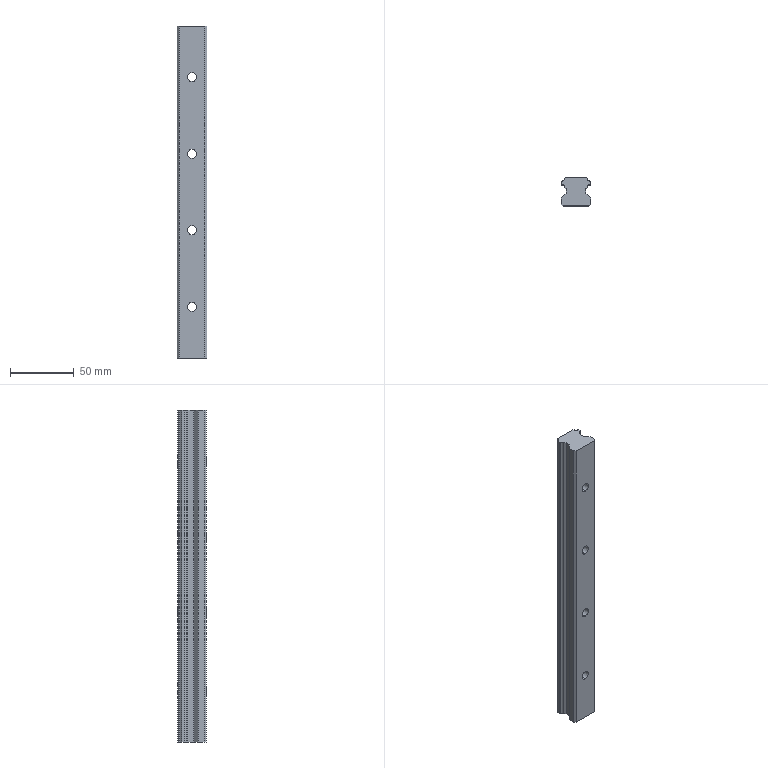Part | SolidWorks | features ICE 2, BaseBody 1, HoleWzd 1, LPattern 1 | 1 solid | 48 faces | box 23 x 22 x 260 mm | volume 107500 mm3 | plane 26 | cylinder 22 | commonest cylinder face diameters 7 x8 11 x8 3.5 x6
STEP:
#1=CARTESIAN_POINT('',(0.,-9.,-134.5));
#2=VERTEX_POINT('',#1);
#3=CARTESIAN_POINT('',(0.,-9.,-123.5));
#4=VERTEX_POINT('',#3);
#5=CARTESIAN_POINT('',(0.,-9.,-129.));
#6=DIRECTION('',(0.,1.,0.));
#7=DIRECTION('',(0.,0.,1.));
#8=AXIS2_PLACEMENT_3D('',#5,#6,#7);
#9=CIRCLE('',#8,5.5);
#10=EDGE_CURVE('',#2,#4,#9,.T.);
#11=ORIENTED_EDGE('',*,*,#10,.F.);
#12=CARTESIAN_POINT('',(0.,0.,-134.5));
#13=VERTEX_POINT('',#12);
#14=CARTESIAN_POINT('',(0.,0.,-134.5));
#15=DIRECTION('',(0.,1.,0.));
#16=VECTOR('',#15,1000.);
#17=LINE('',#14,#16);
#18=EDGE_CURVE('',#2,#13,#17,.T.);
#19=ORIENTED_EDGE('',*,*,#18,.T.);
#20=CARTESIAN_POINT('',(0.,0.,-123.5));
#21=VERTEX_POINT('',#20);
#22=CARTESIAN_POINT('',(0.,0.,-129.));
#23=DIRECTION('',(0.,1.,0.));
#24=DIRECTION('',(0.,0.,1.));
#25=AXIS2_PLACEMENT_3D('',#22,#23,#24);
#26=CIRCLE('',#25,5.5);
#27=EDGE_CURVE('',#13,#21,#26,.T.);
#28=ORIENTED_EDGE('',*,*,#27,.T.);
#29=CARTESIAN_POINT('',(0.,0.,-123.5));
#30=DIRECTION('',(0.,1.,0.));
#31=VECTOR('',#30,1000.);
#32=LINE('',#29,#31);
#33=EDGE_CURVE('',#4,#21,#32,.T.);
#34=ORIENTED_EDGE('',*,*,#33,.F.);
#35=EDGE_LOOP('',(#11,#19,#28,#34));
#36=FACE_OUTER_BOUND('',#35,.T.);
#37=CARTESIAN_POINT('',(0.,0.,-129.));
#38=DIRECTION('',(0.,1.,0.));
#39=DIRECTION('',(0.,0.,1.));
#40=AXIS2_PLACEMENT_3D('',#37,#38,#39);
#41=CYLINDRICAL_SURFACE('',#40,5.5);
#42=ADVANCED_FACE('',(#36),#41,.F.);
#43=CARTESIAN_POINT('',(0.,-22.,-125.5));
#44=VERTEX_POINT('',#43);
#45=CARTESIAN_POINT('',(0.,-22.,-132.5));
#46=VERTEX_POINT('',#45);
#47=CARTESIAN_POINT('',(0.,-22.,-129.));
#48=DIRECTION('',(0.,-1.,0.));
#49=DIRECTION('',(0.,0.,-1.));
#50=AXIS2_PLACEMENT_3D('',#47,#48,#49);
#51=CIRCLE('',#50,3.5);
#52=EDGE_CURVE('',#44,#46,#51,.T.);
#53=ORIENTED_EDGE('',*,*,#52,.T.);
#54=CARTESIAN_POINT('',(0.,-9.,-132.5));
#55=VERTEX_POINT('',#54);
#56=CARTESIAN_POINT('',(0.,0.,-132.5));
#57=DIRECTION('',(0.,1.,0.));
#58=VECTOR('',#57,1000.);
#59=LINE('',#56,#58);
#60=EDGE_CURVE('',#46,#55,#59,.T.);
#61=ORIENTED_EDGE('',*,*,#60,.T.);
#62=CARTESIAN_POINT('',(0.,-9.,-125.5));
#63=VERTEX_POINT('',#62);
#64=CARTESIAN_POINT('',(0.,-9.,-129.));
#65=DIRECTION('',(0.,1.,0.));
#66=DIRECTION('',(0.,0.,1.));
#67=AXIS2_PLACEMENT_3D('',#64,#65,#66);
#68=CIRCLE('',#67,3.5);
#69=EDGE_CURVE('',#55,#63,#68,.T.);
#70=ORIENTED_EDGE('',*,*,#69,.T.);
#71=CARTESIAN_POINT('',(0.,0.,-125.5));
#72=DIRECTION('',(0.,1.,0.));
#73=VECTOR('',#72,1000.);
#74=LINE('',#71,#73);
#75=EDGE_CURVE('',#44,#63,#74,.T.);
#76=ORIENTED_EDGE('',*,*,#75,.F.);
#77=EDGE_LOOP('',(#53,#61,#70,#76));
#78=FACE_OUTER_BOUND('',#77,.T.);
#79=CARTESIAN_POINT('',(0.,0.,-129.));
#80=DIRECTION('',(0.,1.,0.));
#81=DIRECTION('',(0.,0.,1.));
#82=AXIS2_PLACEMENT_3D('',#79,#80,#81);
#83=CYLINDRICAL_SURFACE('',#82,3.5);
#84=ADVANCED_FACE('',(#78),#83,.F.);
#85=CARTESIAN_POINT('',(0.,-9.,-74.5));
#86=VERTEX_POINT('',#85);
#87=CARTESIAN_POINT('',(0.,-9.,-63.5));
#88=VERTEX_POINT('',#87);
#89=CARTESIAN_POINT('',(0.,-9.,-69.));
#90=DIRECTION('',(0.,1.,0.));
#91=DIRECTION('',(0.,0.,1.));
#92=AXIS2_PLACEMENT_3D('',#89,#90,#91);
#93=CIRCLE('',#92,5.5);
#94=EDGE_CURVE('',#86,#88,#93,.T.);
#95=ORIENTED_EDGE('',*,*,#94,.F.);
#96=CARTESIAN_POINT('',(0.,0.,-74.5));
#97=VERTEX_POINT('',#96);
#98=CARTESIAN_POINT('',(0.,0.,-74.5));
#99=DIRECTION('',(0.,1.,0.));
#100=VECTOR('',#99,1000.);
#101=LINE('',#98,#100);
#102=EDGE_CURVE('',#86,#97,#101,.T.);
#103=ORIENTED_EDGE('',*,*,#102,.T.);
#104=CARTESIAN_POINT('',(0.,0.,-63.5));
#105=VERTEX_POINT('',#104);
#106=CARTESIAN_POINT('',(0.,0.,-69.));
#107=DIRECTION('',(0.,1.,0.));
#108=DIRECTION('',(0.,0.,1.));
#109=AXIS2_PLACEMENT_3D('',#106,#107,#108);
#110=CIRCLE('',#109,5.5);
#111=EDGE_CURVE('',#97,#105,#110,.T.);
#112=ORIENTED_EDGE('',*,*,#111,.T.);
#113=CARTESIAN_POINT('',(0.,0.,-63.5));
#114=DIRECTION('',(0.,1.,0.));
#115=VECTOR('',#114,1000.);
#116=LINE('',#113,#115);
#117=EDGE_CURVE('',#88,#105,#116,.T.);
#118=ORIENTED_EDGE('',*,*,#117,.F.);
#119=EDGE_LOOP('',(#95,#103,#112,#118));
#120=FACE_OUTER_BOUND('',#119,.T.);
#121=CARTESIAN_POINT('',(0.,0.,-69.));
#122=DIRECTION('',(0.,1.,0.));
#123=DIRECTION('',(0.,0.,1.));
#124=AXIS2_PLACEMENT_3D('',#121,#122,#123);
#125=CYLINDRICAL_SURFACE('',#124,5.5);
#126=ADVANCED_FACE('',(#120),#125,.F.);
#127=CARTESIAN_POINT('',(0.,-22.,-65.5));
#128=VERTEX_POINT('',#127);
#129=CARTESIAN_POINT('',(0.,-22.,-72.5));
#130=VERTEX_POINT('',#129);
#131=CARTESIAN_POINT('',(0.,-22.,-69.));
#132=DIRECTION('',(0.,-1.,0.));
#133=DIRECTION('',(0.,0.,-1.));
#134=AXIS2_PLACEMENT_3D('',#131,#132,#133);
#135=CIRCLE('',#134,3.5);
#136=EDGE_CURVE('',#128,#130,#135,.T.);
#137=ORIENTED_EDGE('',*,*,#136,.T.);
#138=CARTESIAN_POINT('',(0.,-9.,-72.5));
#139=VERTEX_POINT('',#138);
#140=CARTESIAN_POINT('',(0.,0.,-72.5));
#141=DIRECTION('',(0.,1.,0.));
#142=VECTOR('',#141,1000.);
#143=LINE('',#140,#142);
#144=EDGE_CURVE('',#130,#139,#143,.T.);
#145=ORIENTED_EDGE('',*,*,#144,.T.);
#146=CARTESIAN_POINT('',(0.,-9.,-65.5));
#147=VERTEX_POINT('',#146);
#148=CARTESIAN_POINT('',(0.,-9.,-69.));
#149=DIRECTION('',(0.,1.,0.));
#150=DIRECTION('',(0.,0.,1.));
#151=AXIS2_PLACEMENT_3D('',#148,#149,#150);
#152=CIRCLE('',#151,3.5);
#153=EDGE_CURVE('',#139,#147,#152,.T.);
#154=ORIENTED_EDGE('',*,*,#153,.T.);
#155=CARTESIAN_POINT('',(0.,0.,-65.5));
#156=DIRECTION('',(0.,1.,0.));
#157=VECTOR('',#156,1000.);
#158=LINE('',#155,#157);
#159=EDGE_CURVE('',#128,#147,#158,.T.);
#160=ORIENTED_EDGE('',*,*,#159,.F.);
#161=EDGE_LOOP('',(#137,#145,#154,#160));
#162=FACE_OUTER_BOUND('',#161,.T.);
#163=CARTESIAN_POINT('',(0.,0.,-69.));
#164=DIRECTION('',(0.,1.,0.));
#165=DIRECTION('',(0.,0.,1.));
#166=AXIS2_PLACEMENT_3D('',#163,#164,#165);
#167=CYLINDRICAL_SURFACE('',#166,3.5);
#168=ADVANCED_FACE('',(#162),#167,.F.);
#169=CARTESIAN_POINT('',(0.,-9.,-5.5));
#170=VERTEX_POINT('',#169);
#171=CARTESIAN_POINT('',(0.,-9.,-12.5));
#172=VERTEX_POINT('',#171);
#173=CARTESIAN_POINT('',(0.,-9.,-9.));
#174=DIRECTION('',(0.,-1.,0.));
#175=DIRECTION('',(0.,0.,-1.));
#176=AXIS2_PLACEMENT_3D('',#173,#174,#175);
#177=CIRCLE('',#176,3.5);
#178=EDGE_CURVE('',#170,#172,#177,.T.);
#179=ORIENTED_EDGE('',*,*,#178,.F.);
#180=CARTESIAN_POINT('',(0.,-22.,-5.5));
#181=VERTEX_POINT('',#180);
#182=CARTESIAN_POINT('',(0.,-22.,-5.5));
#183=DIRECTION('',(0.,-1.,0.));
#184=VECTOR('',#183,1000.);
#185=LINE('',#182,#184);
#186=EDGE_CURVE('',#170,#181,#185,.T.);
#187=ORIENTED_EDGE('',*,*,#186,.T.);
#188=CARTESIAN_POINT('',(0.,-22.,-12.5));
#189=VERTEX_POINT('',#188);
#190=CARTESIAN_POINT('',(0.,-22.,-9.));
#191=DIRECTION('',(0.,1.,0.));
#192=DIRECTION('',(0.,0.,-1.));
#193=AXIS2_PLACEMENT_3D('',#190,#191,#192);
#194=CIRCLE('',#193,3.5);
#195=EDGE_CURVE('',#189,#181,#194,.T.);
#196=ORIENTED_EDGE('',*,*,#195,.F.);
#197=CARTESIAN_POINT('',(0.,-22.,-12.5));
#198=DIRECTION('',(0.,-1.,0.));
#199=VECTOR('',#198,1000.);
#200=LINE('',#197,#199);
#201=EDGE_CURVE('',#172,#189,#200,.T.);
#202=ORIENTED_EDGE('',*,*,#201,.F.);
#203=EDGE_LOOP('',(#179,#187,#196,#202));
#204=FACE_OUTER_BOUND('',#203,.T.);
#205=CARTESIAN_POINT('',(0.,-22.,-9.));
#206=DIRECTION('',(0.,-1.,0.));
#207=DIRECTION('',(0.,0.,-1.));
#208=AXIS2_PLACEMENT_3D('',#205,#206,#207);
#209=CYLINDRICAL_SURFACE('',#208,3.5);
#210=ADVANCED_FACE('',(#204),#209,.F.);
#211=CARTESIAN_POINT('',(0.,-9.,54.5));
#212=VERTEX_POINT('',#211);
#213=CARTESIAN_POINT('',(0.,-9.,47.5));
#214=VERTEX_POINT('',#213);
#215=CARTESIAN_POINT('',(0.,-9.,51.));
#216=DIRECTION('',(0.,-1.,0.));
#217=DIRECTION('',(0.,0.,-1.));
#218=AXIS2_PLACEMENT_3D('',#215,#216,#217);
#219=CIRCLE('',#218,3.5);
#220=EDGE_CURVE('',#212,#214,#219,.T.);
#221=ORIENTED_EDGE('',*,*,#220,.F.);
#222=CARTESIAN_POINT('',(0.,-22.,54.5));
#223=VERTEX_POINT('',#222);
#224=CARTESIAN_POINT('',(0.,-22.,54.5));
#225=DIRECTION('',(0.,-1.,0.));
#226=VECTOR('',#225,1000.);
#227=LINE('',#224,#226);
#228=EDGE_CURVE('',#212,#223,#227,.T.);
#229=ORIENTED_EDGE('',*,*,#228,.T.);
#230=CARTESIAN_POINT('',(0.,-22.,47.5));
#231=VERTEX_POINT('',#230);
#232=CARTESIAN_POINT('',(0.,-22.,51.));
#233=DIRECTION('',(0.,1.,0.));
#234=DIRECTION('',(0.,0.,-1.));
#235=AXIS2_PLACEMENT_3D('',#232,#233,#234);
#236=CIRCLE('',#235,3.5);
#237=EDGE_CURVE('',#231,#223,#236,.T.);
#238=ORIENTED_EDGE('',*,*,#237,.F.);
#239=CARTESIAN_POINT('',(0.,-22.,47.5));
#240=DIRECTION('',(0.,-1.,0.));
#241=VECTOR('',#240,1000.);
#242=LINE('',#239,#241);
#243=EDGE_CURVE('',#214,#231,#242,.T.);
#244=ORIENTED_EDGE('',*,*,#243,.F.);
#245=EDGE_LOOP('',(#221,#229,#238,#244));
#246=FACE_OUTER_BOUND('',#245,.T.);
#247=CARTESIAN_POINT('',(0.,-22.,51.));
#248=DIRECTION('',(0.,-1.,0.));
#249=DIRECTION('',(0.,0.,-1.));
#250=AXIS2_PLACEMENT_3D('',#247,#248,#249);
#251=CYLINDRICAL_SURFACE('',#250,3.5);
#252=ADVANCED_FACE('',(#246),#251,.F.);
#253=CARTESIAN_POINT('',(-9.017,-7.063,-169.));
#254=VERTEX_POINT('',#253);
#255=CARTESIAN_POINT('',(-11.079,-5.341,-169.));
#256=VERTEX_POINT('',#255);
#257=CARTESIAN_POINT('',(-10.767,-7.063,-169.));
#258=DIRECTION('',(0.,0.,1.));
#259=DIRECTION('',(-1.,0.,0.));
#260=AXIS2_PLACEMENT_3D('',#257,#258,#259);
#261=CIRCLE('',#260,1.75);
#262=EDGE_CURVE('',#254,#256,#261,.T.);
#263=ORIENTED_EDGE('',*,*,#262,.F.);
#264=CARTESIAN_POINT('',(-9.017,-7.063,91.));
#265=VERTEX_POINT('',#264);
#266=CARTESIAN_POINT('',(-9.017,-7.063,71.));
#267=DIRECTION('',(0.,0.,1.));
#268=VECTOR('',#267,1000.);
#269=LINE('',#266,#268);
#270=EDGE_CURVE('',#254,#265,#269,.T.);
#271=ORIENTED_EDGE('',*,*,#270,.T.);
#272=CARTESIAN_POINT('',(-11.079,-5.341,91.));
#273=VERTEX_POINT('',#272);
#274=CARTESIAN_POINT('',(-10.767,-7.063,91.));
#275=DIRECTION('',(0.,0.,-1.));
#276=DIRECTION('',(1.,0.,0.));
#277=AXIS2_PLACEMENT_3D('',#274,#275,#276);
#278=CIRCLE('',#277,1.75);
#279=EDGE_CURVE('',#273,#265,#278,.T.);
#280=ORIENTED_EDGE('',*,*,#279,.F.);
#281=CARTESIAN_POINT('',(-11.079,-5.341,71.));
#282=DIRECTION('',(0.,0.,1.));
#283=VECTOR('',#282,1000.);
#284=LINE('',#281,#283);
#285=EDGE_CURVE('',#256,#273,#284,.T.);
#286=ORIENTED_EDGE('',*,*,#285,.F.);
#287=EDGE_LOOP('',(#263,#271,#280,#286));
#288=FACE_OUTER_BOUND('',#287,.T.);
#289=CARTESIAN_POINT('',(-10.767,-7.063,71.));
#290=DIRECTION('',(0.,0.,1.));
#291=DIRECTION('',(1.,0.,0.));
#292=AXIS2_PLACEMENT_3D('',#289,#290,#291);
#293=CYLINDRICAL_SURFACE('',#292,1.75);
#294=ADVANCED_FACE('',(#288),#293,.F.);
#295=CARTESIAN_POINT('',(-9.022,-0.9324,-169.));
#296=VERTEX_POINT('',#295);
#297=CARTESIAN_POINT('',(-9.047,-0.6384,-169.));
#298=VERTEX_POINT('',#297);
#299=CARTESIAN_POINT('',(-10.772,-0.9324,-169.));
#300=DIRECTION('',(0.,0.,1.));
#301=DIRECTION('',(-1.,0.,0.));
#302=AXIS2_PLACEMENT_3D('',#299,#300,#301);
#303=CIRCLE('',#302,1.75);
#304=EDGE_CURVE('',#296,#298,#303,.T.);
#305=ORIENTED_EDGE('',*,*,#304,.F.);
#306=CARTESIAN_POINT('',(-9.022,-0.9324,91.));
#307=VERTEX_POINT('',#306);
#308=CARTESIAN_POINT('',(-9.022,-0.9324,71.));
#309=DIRECTION('',(0.,0.,1.));
#310=VECTOR('',#309,1000.);
#311=LINE('',#308,#310);
#312=EDGE_CURVE('',#296,#307,#311,.T.);
#313=ORIENTED_EDGE('',*,*,#312,.T.);
#314=CARTESIAN_POINT('',(-9.047,-0.6384,91.));
#315=VERTEX_POINT('',#314);
#316=CARTESIAN_POINT('',(-10.772,-0.9324,91.));
#317=DIRECTION('',(0.,0.,-1.));
#318=DIRECTION('',(1.,0.,0.));
#319=AXIS2_PLACEMENT_3D('',#316,#317,#318);
#320=CIRCLE('',#319,1.75);
#321=EDGE_CURVE('',#315,#307,#320,.T.);
#322=ORIENTED_EDGE('',*,*,#321,.F.);
#323=CARTESIAN_POINT('',(-9.047,-0.6384,71.));
#324=DIRECTION('',(0.,0.,1.));
#325=VECTOR('',#324,1000.);
#326=LINE('',#323,#325);
#327=EDGE_CURVE('',#298,#315,#326,.T.);
#328=ORIENTED_EDGE('',*,*,#327,.F.);
#329=EDGE_LOOP('',(#305,#313,#322,#328));
#330=FACE_OUTER_BOUND('',#329,.T.);
#331=CARTESIAN_POINT('',(-10.772,-0.9324,71.));
#332=DIRECTION('',(0.,0.,1.));
#333=DIRECTION('',(1.,0.,0.));
#334=AXIS2_PLACEMENT_3D('',#331,#332,#333);
#335=CYLINDRICAL_SURFACE('',#334,1.75);
#336=ADVANCED_FACE('',(#330),#335,.F.);
#337=CARTESIAN_POINT('',(0.,-9.,-14.5));
#338=VERTEX_POINT('',#337);
#339=CARTESIAN_POINT('',(0.,-9.,-3.5));
#340=VERTEX_POINT('',#339);
#341=CARTESIAN_POINT('',(0.,-9.,-9.));
#342=DIRECTION('',(0.,1.,0.));
#343=DIRECTION('',(0.,0.,1.));
#344=AXIS2_PLACEMENT_3D('',#341,#342,#343);
#345=CIRCLE('',#344,5.5);
#346=EDGE_CURVE('',#338,#340,#345,.T.);
#347=ORIENTED_EDGE('',*,*,#346,.F.);
#348=CARTESIAN_POINT('',(0.,0.,-14.5));
#349=VERTEX_POINT('',#348);
#350=CARTESIAN_POINT('',(0.,0.,-14.5));
#351=DIRECTION('',(0.,1.,0.));
#352=VECTOR('',#351,1000.);
#353=LINE('',#350,#352);
#354=EDGE_CURVE('',#338,#349,#353,.T.);
#355=ORIENTED_EDGE('',*,*,#354,.T.);
#356=CARTESIAN_POINT('',(0.,0.,-3.5));
#357=VERTEX_POINT('',#356);
#358=CARTESIAN_POINT('',(0.,0.,-9.));
#359=DIRECTION('',(0.,-1.,0.));
#360=DIRECTION('',(0.,0.,1.));
#361=AXIS2_PLACEMENT_3D('',#358,#359,#360);
#362=CIRCLE('',#361,5.5);
#363=EDGE_CURVE('',#357,#349,#362,.T.);
#364=ORIENTED_EDGE('',*,*,#363,.F.);
#365=CARTESIAN_POINT('',(0.,0.,-3.5));
#366=DIRECTION('',(0.,1.,0.));
#367=VECTOR('',#366,1000.);
#368=LINE('',#365,#367);
#369=EDGE_CURVE('',#340,#357,#368,.T.);
#370=ORIENTED_EDGE('',*,*,#369,.F.);
#371=EDGE_LOOP('',(#347,#355,#364,#370));
#372=FACE_OUTER_BOUND('',#371,.T.);
#373=CARTESIAN_POINT('',(0.,0.,-9.));
#374=DIRECTION('',(0.,1.,0.));
#375=DIRECTION('',(0.,0.,1.));
#376=AXIS2_PLACEMENT_3D('',#373,#374,#375);
#377=CYLINDRICAL_SURFACE('',#376,5.5);
#378=ADVANCED_FACE('',(#372),#377,.F.);
#379=CARTESIAN_POINT('',(0.,-9.,45.5));
#380=VERTEX_POINT('',#379);
#381=CARTESIAN_POINT('',(0.,-9.,56.5));
#382=VERTEX_POINT('',#381);
#383=CARTESIAN_POINT('',(0.,-9.,51.));
#384=DIRECTION('',(0.,1.,0.));
#385=DIRECTION('',(0.,0.,1.));
#386=AXIS2_PLACEMENT_3D('',#383,#384,#385);
#387=CIRCLE('',#386,5.5);
#388=EDGE_CURVE('',#380,#382,#387,.T.);
#389=ORIENTED_EDGE('',*,*,#388,.F.);
#390=CARTESIAN_POINT('',(0.,0.,45.5));
#391=VERTEX_POINT('',#390);
#392=CARTESIAN_POINT('',(0.,0.,45.5));
#393=DIRECTION('',(0.,1.,0.));
#394=VECTOR('',#393,1000.);
#395=LINE('',#392,#394);
#396=EDGE_CURVE('',#380,#391,#395,.T.);
#397=ORIENTED_EDGE('',*,*,#396,.T.);
#398=CARTESIAN_POINT('',(0.,0.,56.5));
#399=VERTEX_POINT('',#398);
#400=CARTESIAN_POINT('',(0.,0.,51.));
#401=DIRECTION('',(0.,-1.,0.));
#402=DIRECTION('',(0.,0.,1.));
#403=AXIS2_PLACEMENT_3D('',#400,#401,#402);
#404=CIRCLE('',#403,5.5);
#405=EDGE_CURVE('',#399,#391,#404,.T.);
#406=ORIENTED_EDGE('',*,*,#405,.F.);
#407=CARTESIAN_POINT('',(0.,0.,56.5));
#408=DIRECTION('',(0.,1.,0.));
#409=VECTOR('',#408,1000.);
#410=LINE('',#407,#409);
#411=EDGE_CURVE('',#382,#399,#410,.T.);
#412=ORIENTED_EDGE('',*,*,#411,.F.);
#413=EDGE_LOOP('',(#389,#397,#406,#412));
#414=FACE_OUTER_BOUND('',#413,.T.);
#415=CARTESIAN_POINT('',(0.,0.,51.));
#416=DIRECTION('',(0.,1.,0.));
#417=DIRECTION('',(0.,0.,1.));
#418=AXIS2_PLACEMENT_3D('',#415,#416,#417);
#419=CYLINDRICAL_SURFACE('',#418,5.5);
#420=ADVANCED_FACE('',(#414),#419,.F.);
#421=ORIENTED_EDGE('',*,*,#52,.F.);
#422=CARTESIAN_POINT('',(0.,-22.,-129.));
#423=DIRECTION('',(0.,-1.,0.));
#424=DIRECTION('',(0.,0.,-1.));
#425=AXIS2_PLACEMENT_3D('',#422,#423,#424);
#426=CIRCLE('',#425,3.5);
#427=EDGE_CURVE('',#46,#44,#426,.T.);
#428=ORIENTED_EDGE('',*,*,#427,.F.);
#429=EDGE_LOOP('',(#421,#428));
#430=FACE_BOUND('',#429,.T.);
#431=ORIENTED_EDGE('',*,*,#136,.F.);
#432=CARTESIAN_POINT('',(0.,-22.,-69.));
#433=DIRECTION('',(0.,-1.,0.));
#434=DIRECTION('',(0.,0.,-1.));
#435=AXIS2_PLACEMENT_3D('',#432,#433,#434);
#436=CIRCLE('',#435,3.5);
#437=EDGE_CURVE('',#130,#128,#436,.T.);
#438=ORIENTED_EDGE('',*,*,#437,.F.);
#439=EDGE_LOOP('',(#431,#438));
#440=FACE_BOUND('',#439,.T.);
#441=ORIENTED_EDGE('',*,*,#195,.T.);
#442=CARTESIAN_POINT('',(0.,-22.,-9.));
#443=DIRECTION('',(0.,1.,0.));
#444=DIRECTION('',(0.,0.,-1.));
#445=AXIS2_PLACEMENT_3D('',#442,#443,#444);
#446=CIRCLE('',#445,3.5);
#447=EDGE_CURVE('',#181,#189,#446,.T.);
#448=ORIENTED_EDGE('',*,*,#447,.T.);
#449=EDGE_LOOP('',(#441,#448));
#450=FACE_BOUND('',#449,.T.);
#451=ORIENTED_EDGE('',*,*,#237,.T.);
#452=CARTESIAN_POINT('',(0.,-22.,51.));
#453=DIRECTION('',(0.,1.,0.));
#454=DIRECTION('',(0.,0.,-1.));
#455=AXIS2_PLACEMENT_3D('',#452,#453,#454);
#456=CIRCLE('',#455,3.5);
#457=EDGE_CURVE('',#223,#231,#456,.T.);
#458=ORIENTED_EDGE('',*,*,#457,.T.);
#459=EDGE_LOOP('',(#451,#458));
#460=FACE_BOUND('',#459,.T.);
#461=CARTESIAN_POINT('',(-10.,-22.,91.));
#462=VERTEX_POINT('',#461);
#463=CARTESIAN_POINT('',(-10.,-22.,-169.));
#464=VERTEX_POINT('',#463);
#465=CARTESIAN_POINT('',(-10.,-22.,-129.));
#466=DIRECTION('',(0.,0.,-1.));
#467=VECTOR('',#466,1000.);
#468=LINE('',#465,#467);
#469=EDGE_CURVE('',#462,#464,#468,.T.);
#470=ORIENTED_EDGE('',*,*,#469,.T.);
#471=CARTESIAN_POINT('',(10.,-22.,-169.));
#472=VERTEX_POINT('',#471);
#473=CARTESIAN_POINT('',(10.,-22.,-169.));
#474=DIRECTION('',(-1.,0.,0.));
#475=VECTOR('',#474,1000.);
#476=LINE('',#473,#475);
#477=EDGE_CURVE('',#472,#464,#476,.T.);
#478=ORIENTED_EDGE('',*,*,#477,.F.);
#479=CARTESIAN_POINT('',(10.,-22.,91.));
#480=VERTEX_POINT('',#479);
#481=CARTESIAN_POINT('',(10.,-22.,-129.));
#482=DIRECTION('',(0.,0.,1.));
#483=VECTOR('',#482,1000.);
#484=LINE('',#481,#483);
#485=EDGE_CURVE('',#472,#480,#484,.T.);
#486=ORIENTED_EDGE('',*,*,#485,.T.);
#487=CARTESIAN_POINT('',(-10.,-22.,91.));
#488=DIRECTION('',(1.,0.,0.));
#489=VECTOR('',#488,1000.);
#490=LINE('',#487,#489);
#491=EDGE_CURVE('',#462,#480,#490,.T.);
#492=ORIENTED_EDGE('',*,*,#491,.F.);
#493=EDGE_LOOP('',(#470,#478,#486,#492));
#494=FACE_OUTER_BOUND('',#493,.T.);
#495=CARTESIAN_POINT('',(-10.,-22.,-129.));
#496=DIRECTION('',(0.,-1.,0.));
#497=DIRECTION('',(0.,0.,-1.));
#498=AXIS2_PLACEMENT_3D('',#495,#496,#497);
#499=PLANE('',#498);
#500=ADVANCED_FACE('',(#430,#440,#450,#460,#494),#499,.T.);
#501=ORIENTED_EDGE('',*,*,#186,.F.);
#502=CARTESIAN_POINT('',(0.,-9.,-9.));
#503=DIRECTION('',(0.,-1.,0.));
#504=DIRECTION('',(0.,0.,-1.));
#505=AXIS2_PLACEMENT_3D('',#502,#503,#504);
#506=CIRCLE('',#505,3.5);
#507=EDGE_CURVE('',#172,#170,#506,.T.);
#508=ORIENTED_EDGE('',*,*,#507,.F.);
#509=ORIENTED_EDGE('',*,*,#201,.T.);
#510=ORIENTED_EDGE('',*,*,#447,.F.);
#511=EDGE_LOOP('',(#501,#508,#509,#510));
#512=FACE_OUTER_BOUND('',#511,.T.);
#513=CARTESIAN_POINT('',(0.,-22.,-9.));
#514=DIRECTION('',(0.,-1.,0.));
#515=DIRECTION('',(0.,0.,-1.));
#516=AXIS2_PLACEMENT_3D('',#513,#514,#515);
#517=CYLINDRICAL_SURFACE('',#516,3.5);
#518=ADVANCED_FACE('',(#512),#517,.F.);
#519=ORIENTED_EDGE('',*,*,#228,.F.);
#520=CARTESIAN_POINT('',(0.,-9.,51.));
#521=DIRECTION('',(0.,-1.,0.));
#522=DIRECTION('',(0.,0.,-1.));
#523=AXIS2_PLACEMENT_3D('',#520,#521,#522);
#524=CIRCLE('',#523,3.5);
#525=EDGE_CURVE('',#214,#212,#524,.T.);
#526=ORIENTED_EDGE('',*,*,#525,.F.);
#527=ORIENTED_EDGE('',*,*,#243,.T.);
#528=ORIENTED_EDGE('',*,*,#457,.F.);
#529=EDGE_LOOP('',(#519,#526,#527,#528));
#530=FACE_OUTER_BOUND('',#529,.T.);
#531=CARTESIAN_POINT('',(0.,-22.,51.));
#532=DIRECTION('',(0.,-1.,0.));
#533=DIRECTION('',(0.,0.,-1.));
#534=AXIS2_PLACEMENT_3D('',#531,#532,#533);
#535=CYLINDRICAL_SURFACE('',#534,3.5);
#536=ADVANCED_FACE('',(#530),#535,.F.);
#537=CARTESIAN_POINT('',(-11.5,-20.5,91.));
#538=VERTEX_POINT('',#537);
#539=CARTESIAN_POINT('',(-11.5,-20.5,-169.));
#540=VERTEX_POINT('',#539);
#541=CARTESIAN_POINT('',(-11.5,-20.5,-129.));
#542=DIRECTION('',(0.,0.,-1.));
#543=VECTOR('',#542,1000.);
#544=LINE('',#541,#543);
#545=EDGE_CURVE('',#538,#540,#544,.T.);
#546=ORIENTED_EDGE('',*,*,#545,.T.);
#547=CARTESIAN_POINT('',(-10.,-22.,-169.));
#548=DIRECTION('',(-0.7071,0.7071,0.));
#549=VECTOR('',#548,1000.);
#550=LINE('',#547,#549);
#551=EDGE_CURVE('',#464,#540,#550,.T.);
#552=ORIENTED_EDGE('',*,*,#551,.F.);
#553=ORIENTED_EDGE('',*,*,#469,.F.);
#554=CARTESIAN_POINT('',(-11.5,-20.5,91.));
#555=DIRECTION('',(0.7071,-0.7071,0.));
#556=VECTOR('',#555,1000.);
#557=LINE('',#554,#556);
#558=EDGE_CURVE('',#538,#462,#557,.T.);
#559=ORIENTED_EDGE('',*,*,#558,.F.);
#560=EDGE_LOOP('',(#546,#552,#553,#559));
#561=FACE_OUTER_BOUND('',#560,.T.);
#562=CARTESIAN_POINT('',(-11.5,-20.5,-129.));
#563=DIRECTION('',(-0.7071,-0.7071,0.));
#564=DIRECTION('',(0.7071,-0.7071,0.));
#565=AXIS2_PLACEMENT_3D('',#562,#563,#564);
#566=PLANE('',#565);
#567=ADVANCED_FACE('',(#561),#566,.T.);
#568=ORIENTED_EDGE('',*,*,#485,.F.);
#569=CARTESIAN_POINT('',(11.5,-20.5,-169.));
#570=VERTEX_POINT('',#569);
#571=CARTESIAN_POINT('',(11.5,-20.5,-169.));
#572=DIRECTION('',(-0.7071,-0.7071,0.));
#573=VECTOR('',#572,1000.);
#574=LINE('',#571,#573);
#575=EDGE_CURVE('',#570,#472,#574,.T.);
#576=ORIENTED_EDGE('',*,*,#575,.F.);
#577=CARTESIAN_POINT('',(11.5,-20.5,91.));
#578=VERTEX_POINT('',#577);
#579=CARTESIAN_POINT('',(11.5,-20.5,-129.));
#580=DIRECTION('',(0.,0.,1.));
#581=VECTOR('',#580,1000.);
#582=LINE('',#579,#581);
#583=EDGE_CURVE('',#570,#578,#582,.T.);
#584=ORIENTED_EDGE('',*,*,#583,.T.);
#585=CARTESIAN_POINT('',(10.,-22.,91.));
#586=DIRECTION('',(0.7071,0.7071,0.));
#587=VECTOR('',#586,1000.);
#588=LINE('',#585,#587);
#589=EDGE_CURVE('',#480,#578,#588,.T.);
#590=ORIENTED_EDGE('',*,*,#589,.F.);
#591=EDGE_LOOP('',(#568,#576,#584,#590));
#592=FACE_OUTER_BOUND('',#591,.T.);
#593=CARTESIAN_POINT('',(10.,-22.,-129.));
#594=DIRECTION('',(0.7071,-0.7071,0.));
#595=DIRECTION('',(0.7071,0.7071,0.));
#596=AXIS2_PLACEMENT_3D('',#593,#594,#595);
#597=PLANE('',#596);
#598=ADVANCED_FACE('',(#592),#597,.T.);
#599=ORIENTED_EDGE('',*,*,#507,.T.);
#600=ORIENTED_EDGE('',*,*,#178,.T.);
#601=EDGE_LOOP('',(#599,#600));
#602=FACE_BOUND('',#601,.T.);
#603=CARTESIAN_POINT('',(0.,-9.,-9.));
#604=DIRECTION('',(0.,1.,0.));
#605=DIRECTION('',(0.,0.,1.));
#606=AXIS2_PLACEMENT_3D('',#603,#604,#605);
#607=CIRCLE('',#606,5.5);
#608=EDGE_CURVE('',#340,#338,#607,.T.);
#609=ORIENTED_EDGE('',*,*,#608,.T.);
#610=ORIENTED_EDGE('',*,*,#346,.T.);
#611=EDGE_LOOP('',(#609,#610));
#612=FACE_OUTER_BOUND('',#611,.T.);
#613=CARTESIAN_POINT('',(-11.5,-9.,-129.));
#614=DIRECTION('',(0.,1.,0.));
#615=DIRECTION('',(0.,0.,1.));
#616=AXIS2_PLACEMENT_3D('',#613,#614,#615);
#617=PLANE('',#616);
#618=ADVANCED_FACE('',(#602,#612),#617,.T.);
#619=ORIENTED_EDGE('',*,*,#525,.T.);
#620=ORIENTED_EDGE('',*,*,#220,.T.);
#621=EDGE_LOOP('',(#619,#620));
#622=FACE_BOUND('',#621,.T.);
#623=CARTESIAN_POINT('',(0.,-9.,51.));
#624=DIRECTION('',(0.,1.,0.));
#625=DIRECTION('',(0.,0.,1.));
#626=AXIS2_PLACEMENT_3D('',#623,#624,#625);
#627=CIRCLE('',#626,5.5);
#628=EDGE_CURVE('',#382,#380,#627,.T.);
#629=ORIENTED_EDGE('',*,*,#628,.T.);
#630=ORIENTED_EDGE('',*,*,#388,.T.);
#631=EDGE_LOOP('',(#629,#630));
#632=FACE_OUTER_BOUND('',#631,.T.);
#633=CARTESIAN_POINT('',(-11.5,-9.,-129.));
#634=DIRECTION('',(0.,1.,0.));
#635=DIRECTION('',(0.,0.,1.));
#636=AXIS2_PLACEMENT_3D('',#633,#634,#635);
#637=PLANE('',#636);
#638=ADVANCED_FACE('',(#622,#632),#637,.T.);
#639=CARTESIAN_POINT('',(7.8,-8.62,91.));
#640=VERTEX_POINT('',#639);
#641=CARTESIAN_POINT('',(7.8,-8.62,-169.));
#642=VERTEX_POINT('',#641);
#643=CARTESIAN_POINT('',(7.8,-8.62,-129.));
#644=DIRECTION('',(0.,0.,-1.));
#645=VECTOR('',#644,1000.);
#646=LINE('',#643,#645);
#647=EDGE_CURVE('',#640,#642,#646,.T.);
#648=ORIENTED_EDGE('',*,*,#647,.T.);
#649=CARTESIAN_POINT('',(9.045,-7.375,-169.));
#650=VERTEX_POINT('',#649);
#651=CARTESIAN_POINT('',(9.045,-7.375,-169.));
#652=DIRECTION('',(-0.7071,-0.7071,0.));
#653=VECTOR('',#652,1000.);
#654=LINE('',#651,#653);
#655=EDGE_CURVE('',#650,#642,#654,.T.);
#656=ORIENTED_EDGE('',*,*,#655,.F.);
#657=CARTESIAN_POINT('',(9.045,-7.375,91.));
#658=VERTEX_POINT('',#657);
#659=CARTESIAN_POINT('',(9.045,-7.375,-129.));
#660=DIRECTION('',(0.,0.,1.));
#661=VECTOR('',#660,1000.);
#662=LINE('',#659,#661);
#663=EDGE_CURVE('',#650,#658,#662,.T.);
#664=ORIENTED_EDGE('',*,*,#663,.T.);
#665=CARTESIAN_POINT('',(7.8,-8.62,91.));
#666=DIRECTION('',(0.7071,0.7071,0.));
#667=VECTOR('',#666,1000.);
#668=LINE('',#665,#667);
#669=EDGE_CURVE('',#640,#658,#668,.T.);
#670=ORIENTED_EDGE('',*,*,#669,.F.);
#671=EDGE_LOOP('',(#648,#656,#664,#670));
#672=FACE_OUTER_BOUND('',#671,.T.);
#673=CARTESIAN_POINT('',(7.8,-8.62,-129.));
#674=DIRECTION('',(0.7071,-0.7071,0.));
#675=DIRECTION('',(0.7071,0.7071,0.));
#676=AXIS2_PLACEMENT_3D('',#673,#674,#675);
#677=PLANE('',#676);
#678=ADVANCED_FACE('',(#672),#677,.T.);
#679=CARTESIAN_POINT('',(7.8,-12.201,91.));
#680=VERTEX_POINT('',#679);
#681=CARTESIAN_POINT('',(7.8,-12.201,-169.));
#682=VERTEX_POINT('',#681);
#683=CARTESIAN_POINT('',(7.8,-12.201,-129.));
#684=DIRECTION('',(0.,0.,-1.));
#685=VECTOR('',#684,1000.);
#686=LINE('',#683,#685);
#687=EDGE_CURVE('',#680,#682,#686,.T.);
#688=ORIENTED_EDGE('',*,*,#687,.T.);
#689=CARTESIAN_POINT('',(7.8,-8.62,-169.));
#690=DIRECTION('',(0.,-1.,0.));
#691=VECTOR('',#690,1000.);
#692=LINE('',#689,#691);
#693=EDGE_CURVE('',#642,#682,#692,.T.);
#694=ORIENTED_EDGE('',*,*,#693,.F.);
#695=ORIENTED_EDGE('',*,*,#647,.F.);
#696=CARTESIAN_POINT('',(7.8,-12.201,91.));
#697=DIRECTION('',(0.,1.,0.));
#698=VECTOR('',#697,1000.);
#699=LINE('',#696,#698);
#700=EDGE_CURVE('',#680,#640,#699,.T.);
#701=ORIENTED_EDGE('',*,*,#700,.F.);
#702=EDGE_LOOP('',(#688,#694,#695,#701));
#703=FACE_OUTER_BOUND('',#702,.T.);
#704=CARTESIAN_POINT('',(7.8,-12.201,-129.));
#705=DIRECTION('',(1.,0.,0.));
#706=DIRECTION('',(0.,0.,-1.));
#707=AXIS2_PLACEMENT_3D('',#704,#705,#706);
#708=PLANE('',#707);
#709=ADVANCED_FACE('',(#703),#708,.T.);
#710=CARTESIAN_POINT('',(11.5,-15.901,91.));
#711=VERTEX_POINT('',#710);
#712=CARTESIAN_POINT('',(11.5,-15.901,-169.));
#713=VERTEX_POINT('',#712);
#714=CARTESIAN_POINT('',(11.5,-15.901,-129.));
#715=DIRECTION('',(0.,0.,-1.));
#716=VECTOR('',#715,1000.);
#717=LINE('',#714,#716);
#718=EDGE_CURVE('',#711,#713,#717,.T.);
#719=ORIENTED_EDGE('',*,*,#718,.T.);
#720=CARTESIAN_POINT('',(7.8,-12.201,-169.));
#721=DIRECTION('',(0.7071,-0.7071,0.));
#722=VECTOR('',#721,1000.);
#723=LINE('',#720,#722);
#724=EDGE_CURVE('',#682,#713,#723,.T.);
#725=ORIENTED_EDGE('',*,*,#724,.F.);
#726=ORIENTED_EDGE('',*,*,#687,.F.);
#727=CARTESIAN_POINT('',(11.5,-15.901,91.));
#728=DIRECTION('',(-0.7071,0.7071,0.));
#729=VECTOR('',#728,1000.);
#730=LINE('',#727,#729);
#731=EDGE_CURVE('',#711,#680,#730,.T.);
#732=ORIENTED_EDGE('',*,*,#731,.F.);
#733=EDGE_LOOP('',(#719,#725,#726,#732));
#734=FACE_OUTER_BOUND('',#733,.T.);
#735=CARTESIAN_POINT('',(11.5,-15.901,-129.));
#736=DIRECTION('',(0.7071,0.7071,0.));
#737=DIRECTION('',(-0.7071,0.7071,0.));
#738=AXIS2_PLACEMENT_3D('',#735,#736,#737);
#739=PLANE('',#738);
#740=ADVANCED_FACE('',(#734),#739,.T.);
#741=ORIENTED_EDGE('',*,*,#583,.F.);
#742=CARTESIAN_POINT('',(11.5,-15.901,-169.));
#743=DIRECTION('',(0.,-1.,0.));
#744=VECTOR('',#743,1000.);
#745=LINE('',#742,#744);
#746=EDGE_CURVE('',#713,#570,#745,.T.);
#747=ORIENTED_EDGE('',*,*,#746,.F.);
#748=ORIENTED_EDGE('',*,*,#718,.F.);
#749=CARTESIAN_POINT('',(11.5,-20.5,91.));
#750=DIRECTION('',(0.,1.,0.));
#751=VECTOR('',#750,1000.);
#752=LINE('',#749,#751);
#753=EDGE_CURVE('',#578,#711,#752,.T.);
#754=ORIENTED_EDGE('',*,*,#753,.F.);
#755=EDGE_LOOP('',(#741,#747,#748,#754));
#756=FACE_OUTER_BOUND('',#755,.T.);
#757=CARTESIAN_POINT('',(11.5,-20.5,-129.));
#758=DIRECTION('',(1.,0.,0.));
#759=DIRECTION('',(0.,0.,-1.));
#760=AXIS2_PLACEMENT_3D('',#757,#758,#759);
#761=PLANE('',#760);
#762=ADVANCED_FACE('',(#756),#761,.T.);
#763=CARTESIAN_POINT('',(-11.5,-15.901,91.));
#764=VERTEX_POINT('',#763);
#765=CARTESIAN_POINT('',(-11.5,-15.901,-169.));
#766=VERTEX_POINT('',#765);
#767=CARTESIAN_POINT('',(-11.5,-15.901,-129.));
#768=DIRECTION('',(0.,0.,-1.));
#769=VECTOR('',#768,1000.);
#770=LINE('',#767,#769);
#771=EDGE_CURVE('',#764,#766,#770,.T.);
#772=ORIENTED_EDGE('',*,*,#771,.T.);
#773=CARTESIAN_POINT('',(-11.5,-20.5,-169.));
#774=DIRECTION('',(0.,1.,0.));
#775=VECTOR('',#774,1000.);
#776=LINE('',#773,#775);
#777=EDGE_CURVE('',#540,#766,#776,.T.);
#778=ORIENTED_EDGE('',*,*,#777,.F.);
#779=ORIENTED_EDGE('',*,*,#545,.F.);
#780=CARTESIAN_POINT('',(-11.5,-15.901,91.));
#781=DIRECTION('',(0.,-1.,0.));
#782=VECTOR('',#781,1000.);
#783=LINE('',#780,#782);
#784=EDGE_CURVE('',#764,#538,#783,.T.);
#785=ORIENTED_EDGE('',*,*,#784,.F.);
#786=EDGE_LOOP('',(#772,#778,#779,#785));
#787=FACE_OUTER_BOUND('',#786,.T.);
#788=CARTESIAN_POINT('',(-11.5,-15.901,-129.));
#789=DIRECTION('',(-1.,0.,0.));
#790=DIRECTION('',(0.,0.,1.));
#791=AXIS2_PLACEMENT_3D('',#788,#789,#790);
#792=PLANE('',#791);
#793=ADVANCED_FACE('',(#787),#792,.T.);
#794=CARTESIAN_POINT('',(-7.8,-12.201,91.));
#795=VERTEX_POINT('',#794);
#796=CARTESIAN_POINT('',(-7.8,-12.201,-169.));
#797=VERTEX_POINT('',#796);
#798=CARTESIAN_POINT('',(-7.8,-12.201,-129.));
#799=DIRECTION('',(0.,0.,-1.));
#800=VECTOR('',#799,1000.);
#801=LINE('',#798,#800);
#802=EDGE_CURVE('',#795,#797,#801,.T.);
#803=ORIENTED_EDGE('',*,*,#802,.T.);
#804=CARTESIAN_POINT('',(-11.5,-15.901,-169.));
#805=DIRECTION('',(0.7071,0.7071,0.));
#806=VECTOR('',#805,1000.);
#807=LINE('',#804,#806);
#808=EDGE_CURVE('',#766,#797,#807,.T.);
#809=ORIENTED_EDGE('',*,*,#808,.F.);
#810=ORIENTED_EDGE('',*,*,#771,.F.);
#811=CARTESIAN_POINT('',(-7.8,-12.201,91.));
#812=DIRECTION('',(-0.7071,-0.7071,0.));
#813=VECTOR('',#812,1000.);
#814=LINE('',#811,#813);
#815=EDGE_CURVE('',#795,#764,#814,.T.);
#816=ORIENTED_EDGE('',*,*,#815,.F.);
#817=EDGE_LOOP('',(#803,#809,#810,#816));
#818=FACE_OUTER_BOUND('',#817,.T.);
#819=CARTESIAN_POINT('',(-7.8,-12.201,-129.));
#820=DIRECTION('',(-0.7071,0.7071,0.));
#821=DIRECTION('',(-0.7071,-0.7071,0.));
#822=AXIS2_PLACEMENT_3D('',#819,#820,#821);
#823=PLANE('',#822);
#824=ADVANCED_FACE('',(#818),#823,.T.);
#825=CARTESIAN_POINT('',(-7.8,-8.62,91.));
#826=VERTEX_POINT('',#825);
#827=CARTESIAN_POINT('',(-7.8,-8.62,-169.));
#828=VERTEX_POINT('',#827);
#829=CARTESIAN_POINT('',(-7.8,-8.62,-129.));
#830=DIRECTION('',(0.,0.,-1.));
#831=VECTOR('',#830,1000.);
#832=LINE('',#829,#831);
#833=EDGE_CURVE('',#826,#828,#832,.T.);
#834=ORIENTED_EDGE('',*,*,#833,.T.);
#835=CARTESIAN_POINT('',(-7.8,-12.201,-169.));
#836=DIRECTION('',(0.,1.,0.));
#837=VECTOR('',#836,1000.);
#838=LINE('',#835,#837);
#839=EDGE_CURVE('',#797,#828,#838,.T.);
#840=ORIENTED_EDGE('',*,*,#839,.F.);
#841=ORIENTED_EDGE('',*,*,#802,.F.);
#842=CARTESIAN_POINT('',(-7.8,-8.62,91.));
#843=DIRECTION('',(0.,-1.,0.));
#844=VECTOR('',#843,1000.);
#845=LINE('',#842,#844);
#846=EDGE_CURVE('',#826,#795,#845,.T.);
#847=ORIENTED_EDGE('',*,*,#846,.F.);
#848=EDGE_LOOP('',(#834,#840,#841,#847));
#849=FACE_OUTER_BOUND('',#848,.T.);
#850=CARTESIAN_POINT('',(-7.8,-8.62,-129.));
#851=DIRECTION('',(-1.,0.,0.));
#852=DIRECTION('',(0.,0.,1.));
#853=AXIS2_PLACEMENT_3D('',#850,#851,#852);
#854=PLANE('',#853);
#855=ADVANCED_FACE('',(#849),#854,.T.);
#856=CARTESIAN_POINT('',(-9.045,-7.375,91.));
#857=VERTEX_POINT('',#856);
#858=CARTESIAN_POINT('',(-9.045,-7.375,-169.));
#859=VERTEX_POINT('',#858);
#860=CARTESIAN_POINT('',(-9.045,-7.375,-129.));
#861=DIRECTION('',(0.,0.,-1.));
#862=VECTOR('',#861,1000.);
#863=LINE('',#860,#862);
#864=EDGE_CURVE('',#857,#859,#863,.T.);
#865=ORIENTED_EDGE('',*,*,#864,.T.);
#866=CARTESIAN_POINT('',(-7.8,-8.62,-169.));
#867=DIRECTION('',(-0.7071,0.7071,0.));
#868=VECTOR('',#867,1000.);
#869=LINE('',#866,#868);
#870=EDGE_CURVE('',#828,#859,#869,.T.);
#871=ORIENTED_EDGE('',*,*,#870,.F.);
#872=ORIENTED_EDGE('',*,*,#833,.F.);
#873=CARTESIAN_POINT('',(-9.045,-7.375,91.));
#874=DIRECTION('',(0.7071,-0.7071,0.));
#875=VECTOR('',#874,1000.);
#876=LINE('',#873,#875);
#877=EDGE_CURVE('',#857,#826,#876,.T.);
#878=ORIENTED_EDGE('',*,*,#877,.F.);
#879=EDGE_LOOP('',(#865,#871,#872,#878));
#880=FACE_OUTER_BOUND('',#879,.T.);
#881=CARTESIAN_POINT('',(-9.045,-7.375,-129.));
#882=DIRECTION('',(-0.7071,-0.7071,0.));
#883=DIRECTION('',(0.7071,-0.7071,0.));
#884=AXIS2_PLACEMENT_3D('',#881,#882,#883);
#885=PLANE('',#884);
#886=ADVANCED_FACE('',(#880),#885,.T.);
#887=ORIENTED_EDGE('',*,*,#270,.F.);
#888=CARTESIAN_POINT('',(-10.767,-7.063,-169.));
#889=DIRECTION('',(0.,0.,1.));
#890=DIRECTION('',(-1.,0.,0.));
#891=AXIS2_PLACEMENT_3D('',#888,#889,#890);
#892=CIRCLE('',#891,1.75);
#893=EDGE_CURVE('',#859,#254,#892,.T.);
#894=ORIENTED_EDGE('',*,*,#893,.F.);
#895=ORIENTED_EDGE('',*,*,#864,.F.);
#896=CARTESIAN_POINT('',(-10.767,-7.063,91.));
#897=DIRECTION('',(0.,0.,-1.));
#898=DIRECTION('',(1.,0.,0.));
#899=AXIS2_PLACEMENT_3D('',#896,#897,#898);
#900=CIRCLE('',#899,1.75);
#901=EDGE_CURVE('',#265,#857,#900,.T.);
#902=ORIENTED_EDGE('',*,*,#901,.F.);
#903=EDGE_LOOP('',(#887,#894,#895,#902));
#904=FACE_OUTER_BOUND('',#903,.T.);
#905=CARTESIAN_POINT('',(-10.767,-7.063,71.));
#906=DIRECTION('',(0.,0.,1.));
#907=DIRECTION('',(1.,0.,0.));
#908=AXIS2_PLACEMENT_3D('',#905,#906,#907);
#909=CYLINDRICAL_SURFACE('',#908,1.75);
#910=ADVANCED_FACE('',(#904),#909,.F.);
#911=CARTESIAN_POINT('',(-11.5,-3.091,91.));
#912=VERTEX_POINT('',#911);
#913=CARTESIAN_POINT('',(-11.5,-3.091,-169.));
#914=VERTEX_POINT('',#913);
#915=CARTESIAN_POINT('',(-11.5,-3.091,-129.));
#916=DIRECTION('',(0.,0.,-1.));
#917=VECTOR('',#916,1000.);
#918=LINE('',#915,#917);
#919=EDGE_CURVE('',#912,#914,#918,.T.);
#920=ORIENTED_EDGE('',*,*,#919,.T.);
#921=CARTESIAN_POINT('',(-11.5,-4.92,-169.));
#922=VERTEX_POINT('',#921);
#923=CARTESIAN_POINT('',(-11.5,-4.92,-169.));
#924=DIRECTION('',(0.,1.,0.));
#925=VECTOR('',#924,1000.);
#926=LINE('',#923,#925);
#927=EDGE_CURVE('',#922,#914,#926,.T.);
#928=ORIENTED_EDGE('',*,*,#927,.F.);
#929=CARTESIAN_POINT('',(-11.5,-4.92,91.));
#930=VERTEX_POINT('',#929);
#931=CARTESIAN_POINT('',(-11.5,-4.92,-129.));
#932=DIRECTION('',(0.,0.,1.));
#933=VECTOR('',#932,1000.);
#934=LINE('',#931,#933);
#935=EDGE_CURVE('',#922,#930,#934,.T.);
#936=ORIENTED_EDGE('',*,*,#935,.T.);
#937=CARTESIAN_POINT('',(-11.5,-3.091,91.));
#938=DIRECTION('',(0.,-1.,0.));
#939=VECTOR('',#938,1000.);
#940=LINE('',#937,#939);
#941=EDGE_CURVE('',#912,#930,#940,.T.);
#942=ORIENTED_EDGE('',*,*,#941,.F.);
#943=EDGE_LOOP('',(#920,#928,#936,#942));
#944=FACE_OUTER_BOUND('',#943,.T.);
#945=CARTESIAN_POINT('',(-11.5,-3.091,-129.));
#946=DIRECTION('',(-1.,0.,0.));
#947=DIRECTION('',(0.,0.,1.));
#948=AXIS2_PLACEMENT_3D('',#945,#946,#947);
#949=PLANE('',#948);
#950=ADVANCED_FACE('',(#944),#949,.T.);
#951=ORIENTED_EDGE('',*,*,#312,.F.);
#952=CARTESIAN_POINT('',(-11.066,-2.657,-169.));
#953=VERTEX_POINT('',#952);
#954=CARTESIAN_POINT('',(-10.772,-0.9324,-169.));
#955=DIRECTION('',(0.,0.,1.));
#956=DIRECTION('',(-1.,0.,0.));
#957=AXIS2_PLACEMENT_3D('',#954,#955,#956);
#958=CIRCLE('',#957,1.75);
#959=EDGE_CURVE('',#953,#296,#958,.T.);
#960=ORIENTED_EDGE('',*,*,#959,.F.);
#961=CARTESIAN_POINT('',(-11.066,-2.657,91.));
#962=VERTEX_POINT('',#961);
#963=CARTESIAN_POINT('',(-11.066,-2.657,71.));
#964=DIRECTION('',(0.,0.,-1.));
#965=VECTOR('',#964,1000.);
#966=LINE('',#963,#965);
#967=EDGE_CURVE('',#962,#953,#966,.T.);
#968=ORIENTED_EDGE('',*,*,#967,.F.);
#969=CARTESIAN_POINT('',(-10.772,-0.9324,91.));
#970=DIRECTION('',(0.,0.,-1.));
#971=DIRECTION('',(1.,0.,0.));
#972=AXIS2_PLACEMENT_3D('',#969,#970,#971);
#973=CIRCLE('',#972,1.75);
#974=EDGE_CURVE('',#307,#962,#973,.T.);
#975=ORIENTED_EDGE('',*,*,#974,.F.);
#976=EDGE_LOOP('',(#951,#960,#968,#975));
#977=FACE_OUTER_BOUND('',#976,.T.);
#978=CARTESIAN_POINT('',(-10.772,-0.9324,71.));
#979=DIRECTION('',(0.,0.,1.));
#980=DIRECTION('',(1.,0.,0.));
#981=AXIS2_PLACEMENT_3D('',#978,#979,#980);
#982=CYLINDRICAL_SURFACE('',#981,1.75);
#983=ADVANCED_FACE('',(#977),#982,.F.);
#984=CARTESIAN_POINT('',(0.,0.,-129.));
#985=DIRECTION('',(0.,1.,0.));
#986=DIRECTION('',(0.,0.,1.));
#987=AXIS2_PLACEMENT_3D('',#984,#985,#986);
#988=CIRCLE('',#987,5.5);
#989=EDGE_CURVE('',#21,#13,#988,.T.);
#990=ORIENTED_EDGE('',*,*,#989,.F.);
#991=ORIENTED_EDGE('',*,*,#27,.F.);
#992=EDGE_LOOP('',(#990,#991));
#993=FACE_BOUND('',#992,.T.);
#994=CARTESIAN_POINT('',(0.,0.,-69.));
#995=DIRECTION('',(0.,1.,0.));
#996=DIRECTION('',(0.,0.,1.));
#997=AXIS2_PLACEMENT_3D('',#994,#995,#996);
#998=CIRCLE('',#997,5.5);
#999=EDGE_CURVE('',#105,#97,#998,.T.);
#1000=ORIENTED_EDGE('',*,*,#999,.F.);
#1001=ORIENTED_EDGE('',*,*,#111,.F.);
#1002=EDGE_LOOP('',(#1000,#1001));
#1003=FACE_BOUND('',#1002,.T.);
#1004=ORIENTED_EDGE('',*,*,#363,.T.);
#1005=CARTESIAN_POINT('',(0.,0.,-9.));
#1006=DIRECTION('',(0.,-1.,0.));
#1007=DIRECTION('',(0.,0.,1.));
#1008=AXIS2_PLACEMENT_3D('',#1005,#1006,#1007);
#1009=CIRCLE('',#1008,5.5);
#1010=EDGE_CURVE('',#349,#357,#1009,.T.);
#1011=ORIENTED_EDGE('',*,*,#1010,.T.);
#1012=EDGE_LOOP('',(#1004,#1011));
#1013=FACE_BOUND('',#1012,.T.);
#1014=ORIENTED_EDGE('',*,*,#405,.T.);
#1015=CARTESIAN_POINT('',(0.,0.,51.));
#1016=DIRECTION('',(0.,-1.,0.));
#1017=DIRECTION('',(0.,0.,1.));
#1018=AXIS2_PLACEMENT_3D('',#1015,#1016,#1017);
#1019=CIRCLE('',#1018,5.5);
#1020=EDGE_CURVE('',#391,#399,#1019,.T.);
#1021=ORIENTED_EDGE('',*,*,#1020,.T.);
#1022=EDGE_LOOP('',(#1014,#1021));
#1023=FACE_BOUND('',#1022,.T.);
#1024=CARTESIAN_POINT('',(8.409,0.,91.));
#1025=VERTEX_POINT('',#1024);
#1026=CARTESIAN_POINT('',(8.409,0.,-169.));
#1027=VERTEX_POINT('',#1026);
#1028=CARTESIAN_POINT('',(8.409,0.,-129.));
#1029=DIRECTION('',(0.,0.,-1.));
#1030=VECTOR('',#1029,1000.);
#1031=LINE('',#1028,#1030);
#1032=EDGE_CURVE('',#1025,#1027,#1031,.T.);
#1033=ORIENTED_EDGE('',*,*,#1032,.T.);
#1034=CARTESIAN_POINT('',(-8.409,0.,-169.));
#1035=VERTEX_POINT('',#1034);
#1036=CARTESIAN_POINT('',(-8.409,0.,-169.));
#1037=DIRECTION('',(1.,0.,0.));
#1038=VECTOR('',#1037,1000.);
#1039=LINE('',#1036,#1038);
#1040=EDGE_CURVE('',#1035,#1027,#1039,.T.);
#1041=ORIENTED_EDGE('',*,*,#1040,.F.);
#1042=CARTESIAN_POINT('',(-8.409,0.,91.));
#1043=VERTEX_POINT('',#1042);
#1044=CARTESIAN_POINT('',(-8.409,0.,-129.));
#1045=DIRECTION('',(0.,0.,1.));
#1046=VECTOR('',#1045,1000.);
#1047=LINE('',#1044,#1046);
#1048=EDGE_CURVE('',#1035,#1043,#1047,.T.);
#1049=ORIENTED_EDGE('',*,*,#1048,.T.);
#1050=CARTESIAN_POINT('',(8.409,0.,91.));
#1051=DIRECTION('',(-1.,0.,0.));
#1052=VECTOR('',#1051,1000.);
#1053=LINE('',#1050,#1052);
#1054=EDGE_CURVE('',#1025,#1043,#1053,.T.);
#1055=ORIENTED_EDGE('',*,*,#1054,.F.);
#1056=EDGE_LOOP('',(#1033,#1041,#1049,#1055));
#1057=FACE_OUTER_BOUND('',#1056,.T.);
#1058=CARTESIAN_POINT('',(8.409,0.,-129.));
#1059=DIRECTION('',(0.,1.,0.));
#1060=DIRECTION('',(0.,0.,1.));
#1061=AXIS2_PLACEMENT_3D('',#1058,#1059,#1060);
#1062=PLANE('',#1061);
#1063=ADVANCED_FACE('',(#993,#1003,#1013,#1023,#1057),#1062,.T.);
#1064=CARTESIAN_POINT('',(9.047,-0.6384,91.));
#1065=VERTEX_POINT('',#1064);
#1066=CARTESIAN_POINT('',(9.047,-0.6384,-169.));
#1067=VERTEX_POINT('',#1066);
#1068=CARTESIAN_POINT('',(9.047,-0.6384,71.));
#1069=DIRECTION('',(0.,0.,-1.));
#1070=VECTOR('',#1069,1000.);
#1071=LINE('',#1068,#1070);
#1072=EDGE_CURVE('',#1065,#1067,#1071,.T.);
#1073=ORIENTED_EDGE('',*,*,#1072,.F.);
#1074=CARTESIAN_POINT('',(11.066,-2.657,91.));
#1075=VERTEX_POINT('',#1074);
#1076=CARTESIAN_POINT('',(10.772,-0.9324,91.));
#1077=DIRECTION('',(0.,0.,-1.));
#1078=DIRECTION('',(1.,0.,0.));
#1079=AXIS2_PLACEMENT_3D('',#1076,#1077,#1078);
#1080=CIRCLE('',#1079,1.75);
#1081=EDGE_CURVE('',#1075,#1065,#1080,.T.);
#1082=ORIENTED_EDGE('',*,*,#1081,.F.);
#1083=CARTESIAN_POINT('',(11.066,-2.657,-169.));
#1084=VERTEX_POINT('',#1083);
#1085=CARTESIAN_POINT('',(11.066,-2.657,71.));
#1086=DIRECTION('',(0.,0.,1.));
#1087=VECTOR('',#1086,1000.);
#1088=LINE('',#1085,#1087);
#1089=EDGE_CURVE('',#1084,#1075,#1088,.T.);
#1090=ORIENTED_EDGE('',*,*,#1089,.F.);
#1091=CARTESIAN_POINT('',(10.772,-0.9324,-169.));
#1092=DIRECTION('',(0.,0.,1.));
#1093=DIRECTION('',(-1.,0.,0.));
#1094=AXIS2_PLACEMENT_3D('',#1091,#1092,#1093);
#1095=CIRCLE('',#1094,1.75);
#1096=EDGE_CURVE('',#1067,#1084,#1095,.T.);
#1097=ORIENTED_EDGE('',*,*,#1096,.F.);
#1098=EDGE_LOOP('',(#1073,#1082,#1090,#1097));
#1099=FACE_OUTER_BOUND('',#1098,.T.);
#1100=CARTESIAN_POINT('',(10.772,-0.9324,71.));
#1101=DIRECTION('',(0.,0.,1.));
#1102=DIRECTION('',(1.,0.,0.));
#1103=AXIS2_PLACEMENT_3D('',#1100,#1101,#1102);
#1104=CYLINDRICAL_SURFACE('',#1103,1.75);
#1105=ADVANCED_FACE('',(#1099),#1104,.F.);
#1106=CARTESIAN_POINT('',(11.5,-4.92,91.));
#1107=VERTEX_POINT('',#1106);
#1108=CARTESIAN_POINT('',(11.5,-4.92,-169.));
#1109=VERTEX_POINT('',#1108);
#1110=CARTESIAN_POINT('',(11.5,-4.92,-129.));
#1111=DIRECTION('',(0.,0.,-1.));
#1112=VECTOR('',#1111,1000.);
#1113=LINE('',#1110,#1112);
#1114=EDGE_CURVE('',#1107,#1109,#1113,.T.);
#1115=ORIENTED_EDGE('',*,*,#1114,.T.);
#1116=CARTESIAN_POINT('',(11.5,-3.091,-169.));
#1117=VERTEX_POINT('',#1116);
#1118=CARTESIAN_POINT('',(11.5,-3.091,-169.));
#1119=DIRECTION('',(0.,-1.,0.));
#1120=VECTOR('',#1119,1000.);
#1121=LINE('',#1118,#1120);
#1122=EDGE_CURVE('',#1117,#1109,#1121,.T.);
#1123=ORIENTED_EDGE('',*,*,#1122,.F.);
#1124=CARTESIAN_POINT('',(11.5,-3.091,91.));
#1125=VERTEX_POINT('',#1124);
#1126=CARTESIAN_POINT('',(11.5,-3.091,-129.));
#1127=DIRECTION('',(0.,0.,1.));
#1128=VECTOR('',#1127,1000.);
#1129=LINE('',#1126,#1128);
#1130=EDGE_CURVE('',#1117,#1125,#1129,.T.);
#1131=ORIENTED_EDGE('',*,*,#1130,.T.);
#1132=CARTESIAN_POINT('',(11.5,-4.92,91.));
#1133=DIRECTION('',(0.,1.,0.));
#1134=VECTOR('',#1133,1000.);
#1135=LINE('',#1132,#1134);
#1136=EDGE_CURVE('',#1107,#1125,#1135,.T.);
#1137=ORIENTED_EDGE('',*,*,#1136,.F.);
#1138=EDGE_LOOP('',(#1115,#1123,#1131,#1137));
#1139=FACE_OUTER_BOUND('',#1138,.T.);
#1140=CARTESIAN_POINT('',(11.5,-4.92,-129.));
#1141=DIRECTION('',(1.,0.,0.));
#1142=DIRECTION('',(0.,0.,-1.));
#1143=AXIS2_PLACEMENT_3D('',#1140,#1141,#1142);
#1144=PLANE('',#1143);
#1145=ADVANCED_FACE('',(#1139),#1144,.T.);
#1146=CARTESIAN_POINT('',(11.079,-5.341,91.));
#1147=VERTEX_POINT('',#1146);
#1148=CARTESIAN_POINT('',(11.079,-5.341,-169.));
#1149=VERTEX_POINT('',#1148);
#1150=CARTESIAN_POINT('',(11.079,-5.341,71.));
#1151=DIRECTION('',(0.,0.,-1.));
#1152=VECTOR('',#1151,1000.);
#1153=LINE('',#1150,#1152);
#1154=EDGE_CURVE('',#1147,#1149,#1153,.T.);
#1155=ORIENTED_EDGE('',*,*,#1154,.F.);
#1156=CARTESIAN_POINT('',(10.767,-7.063,91.));
#1157=DIRECTION('',(0.,0.,-1.));
#1158=DIRECTION('',(1.,0.,0.));
#1159=AXIS2_PLACEMENT_3D('',#1156,#1157,#1158);
#1160=CIRCLE('',#1159,1.75);
#1161=EDGE_CURVE('',#658,#1147,#1160,.T.);
#1162=ORIENTED_EDGE('',*,*,#1161,.F.);
#1163=ORIENTED_EDGE('',*,*,#663,.F.);
#1164=CARTESIAN_POINT('',(10.767,-7.063,-169.));
#1165=DIRECTION('',(0.,0.,1.));
#1166=DIRECTION('',(-1.,0.,0.));
#1167=AXIS2_PLACEMENT_3D('',#1164,#1165,#1166);
#1168=CIRCLE('',#1167,1.75);
#1169=EDGE_CURVE('',#1149,#650,#1168,.T.);
#1170=ORIENTED_EDGE('',*,*,#1169,.F.);
#1171=EDGE_LOOP('',(#1155,#1162,#1163,#1170));
#1172=FACE_OUTER_BOUND('',#1171,.T.);
#1173=CARTESIAN_POINT('',(10.767,-7.063,71.));
#1174=DIRECTION('',(0.,0.,1.));
#1175=DIRECTION('',(1.,0.,0.));
#1176=AXIS2_PLACEMENT_3D('',#1173,#1174,#1175);
#1177=CYLINDRICAL_SURFACE('',#1176,1.75);
#1178=ADVANCED_FACE('',(#1172),#1177,.F.);
#1179=ORIENTED_EDGE('',*,*,#354,.F.);
#1180=ORIENTED_EDGE('',*,*,#608,.F.);
#1181=ORIENTED_EDGE('',*,*,#369,.T.);
#1182=ORIENTED_EDGE('',*,*,#1010,.F.);
#1183=EDGE_LOOP('',(#1179,#1180,#1181,#1182));
#1184=FACE_OUTER_BOUND('',#1183,.T.);
#1185=CARTESIAN_POINT('',(0.,0.,-9.));
#1186=DIRECTION('',(0.,1.,0.));
#1187=DIRECTION('',(0.,0.,1.));
#1188=AXIS2_PLACEMENT_3D('',#1185,#1186,#1187);
#1189=CYLINDRICAL_SURFACE('',#1188,5.5);
#1190=ADVANCED_FACE('',(#1184),#1189,.F.);
#1191=ORIENTED_EDGE('',*,*,#396,.F.);
#1192=ORIENTED_EDGE('',*,*,#628,.F.);
#1193=ORIENTED_EDGE('',*,*,#411,.T.);
#1194=ORIENTED_EDGE('',*,*,#1020,.F.);
#1195=EDGE_LOOP('',(#1191,#1192,#1193,#1194));
#1196=FACE_OUTER_BOUND('',#1195,.T.);
#1197=CARTESIAN_POINT('',(0.,0.,51.));
#1198=DIRECTION('',(0.,1.,0.));
#1199=DIRECTION('',(0.,0.,1.));
#1200=AXIS2_PLACEMENT_3D('',#1197,#1198,#1199);
#1201=CYLINDRICAL_SURFACE('',#1200,5.5);
#1202=ADVANCED_FACE('',(#1196),#1201,.F.);
#1203=ORIENTED_EDGE('',*,*,#935,.F.);
#1204=CARTESIAN_POINT('',(-11.079,-5.341,-169.));
#1205=DIRECTION('',(-0.7071,0.7071,0.));
#1206=VECTOR('',#1205,1000.);
#1207=LINE('',#1204,#1206);
#1208=EDGE_CURVE('',#256,#922,#1207,.T.);
#1209=ORIENTED_EDGE('',*,*,#1208,.F.);
#1210=ORIENTED_EDGE('',*,*,#285,.T.);
#1211=CARTESIAN_POINT('',(-11.5,-4.92,91.));
#1212=DIRECTION('',(0.7071,-0.7071,0.));
#1213=VECTOR('',#1212,1000.);
#1214=LINE('',#1211,#1213);
#1215=EDGE_CURVE('',#930,#273,#1214,.T.);
#1216=ORIENTED_EDGE('',*,*,#1215,.F.);
#1217=EDGE_LOOP('',(#1203,#1209,#1210,#1216));
#1218=FACE_OUTER_BOUND('',#1217,.T.);
#1219=CARTESIAN_POINT('',(-11.5,-4.92,-129.));
#1220=DIRECTION('',(-0.7071,-0.7071,0.));
#1221=DIRECTION('',(0.7071,-0.7071,0.));
#1222=AXIS2_PLACEMENT_3D('',#1219,#1220,#1221);
#1223=PLANE('',#1222);
#1224=ADVANCED_FACE('',(#1218),#1223,.T.);
#1225=ORIENTED_EDGE('',*,*,#967,.T.);
#1226=CARTESIAN_POINT('',(-11.5,-3.091,-169.));
#1227=DIRECTION('',(0.7071,0.7071,0.));
#1228=VECTOR('',#1227,1000.);
#1229=LINE('',#1226,#1228);
#1230=EDGE_CURVE('',#914,#953,#1229,.T.);
#1231=ORIENTED_EDGE('',*,*,#1230,.F.);
#1232=ORIENTED_EDGE('',*,*,#919,.F.);
#1233=CARTESIAN_POINT('',(-11.066,-2.657,91.));
#1234=DIRECTION('',(-0.7071,-0.7071,0.));
#1235=VECTOR('',#1234,1000.);
#1236=LINE('',#1233,#1235);
#1237=EDGE_CURVE('',#962,#912,#1236,.T.);
#1238=ORIENTED_EDGE('',*,*,#1237,.F.);
#1239=EDGE_LOOP('',(#1225,#1231,#1232,#1238));
#1240=FACE_OUTER_BOUND('',#1239,.T.);
#1241=CARTESIAN_POINT('',(-11.066,-2.657,-129.));
#1242=DIRECTION('',(-0.7071,0.7071,0.));
#1243=DIRECTION('',(-0.7071,-0.7071,0.));
#1244=AXIS2_PLACEMENT_3D('',#1241,#1242,#1243);
#1245=PLANE('',#1244);
#1246=ADVANCED_FACE('',(#1240),#1245,.T.);
#1247=ORIENTED_EDGE('',*,*,#1048,.F.);
#1248=CARTESIAN_POINT('',(-9.047,-0.6384,-169.));
#1249=DIRECTION('',(0.7071,0.7071,0.));
#1250=VECTOR('',#1249,1000.);
#1251=LINE('',#1248,#1250);
#1252=EDGE_CURVE('',#298,#1035,#1251,.T.);
#1253=ORIENTED_EDGE('',*,*,#1252,.F.);
#1254=ORIENTED_EDGE('',*,*,#327,.T.);
#1255=CARTESIAN_POINT('',(-8.409,0.,91.));
#1256=DIRECTION('',(-0.7071,-0.7071,0.));
#1257=VECTOR('',#1256,1000.);
#1258=LINE('',#1255,#1257);
#1259=EDGE_CURVE('',#1043,#315,#1258,.T.);
#1260=ORIENTED_EDGE('',*,*,#1259,.F.);
#1261=EDGE_LOOP('',(#1247,#1253,#1254,#1260));
#1262=FACE_OUTER_BOUND('',#1261,.T.);
#1263=CARTESIAN_POINT('',(-8.409,0.,-129.));
#1264=DIRECTION('',(-0.7071,0.7071,0.));
#1265=DIRECTION('',(-0.7071,-0.7071,0.));
#1266=AXIS2_PLACEMENT_3D('',#1263,#1264,#1265);
#1267=PLANE('',#1266);
#1268=ADVANCED_FACE('',(#1262),#1267,.T.);
#1269=ORIENTED_EDGE('',*,*,#1072,.T.);
#1270=CARTESIAN_POINT('',(8.409,0.,-169.));
#1271=DIRECTION('',(0.7071,-0.7071,0.));
#1272=VECTOR('',#1271,1000.);
#1273=LINE('',#1270,#1272);
#1274=EDGE_CURVE('',#1027,#1067,#1273,.T.);
#1275=ORIENTED_EDGE('',*,*,#1274,.F.);
#1276=ORIENTED_EDGE('',*,*,#1032,.F.);
#1277=CARTESIAN_POINT('',(9.047,-0.6384,91.));
#1278=DIRECTION('',(-0.7071,0.7071,0.));
#1279=VECTOR('',#1278,1000.);
#1280=LINE('',#1277,#1279);
#1281=EDGE_CURVE('',#1065,#1025,#1280,.T.);
#1282=ORIENTED_EDGE('',*,*,#1281,.F.);
#1283=EDGE_LOOP('',(#1269,#1275,#1276,#1282));
#1284=FACE_OUTER_BOUND('',#1283,.T.);
#1285=CARTESIAN_POINT('',(9.047,-0.6384,-129.));
#1286=DIRECTION('',(0.7071,0.7071,0.));
#1287=DIRECTION('',(-0.7071,0.7071,0.));
#1288=AXIS2_PLACEMENT_3D('',#1285,#1286,#1287);
#1289=PLANE('',#1288);
#1290=ADVANCED_FACE('',(#1284),#1289,.T.);
#1291=ORIENTED_EDGE('',*,*,#1130,.F.);
#1292=CARTESIAN_POINT('',(11.066,-2.657,-169.));
#1293=DIRECTION('',(0.7071,-0.7071,0.));
#1294=VECTOR('',#1293,1000.);
#1295=LINE('',#1292,#1294);
#1296=EDGE_CURVE('',#1084,#1117,#1295,.T.);
#1297=ORIENTED_EDGE('',*,*,#1296,.F.);
#1298=ORIENTED_EDGE('',*,*,#1089,.T.);
#1299=CARTESIAN_POINT('',(11.5,-3.091,91.));
#1300=DIRECTION('',(-0.7071,0.7071,0.));
#1301=VECTOR('',#1300,1000.);
#1302=LINE('',#1299,#1301);
#1303=EDGE_CURVE('',#1125,#1075,#1302,.T.);
#1304=ORIENTED_EDGE('',*,*,#1303,.F.);
#1305=EDGE_LOOP('',(#1291,#1297,#1298,#1304));
#1306=FACE_OUTER_BOUND('',#1305,.T.);
#1307=CARTESIAN_POINT('',(11.5,-3.091,-129.));
#1308=DIRECTION('',(0.7071,0.7071,0.));
#1309=DIRECTION('',(-0.7071,0.7071,0.));
#1310=AXIS2_PLACEMENT_3D('',#1307,#1308,#1309);
#1311=PLANE('',#1310);
#1312=ADVANCED_FACE('',(#1306),#1311,.T.);
#1313=ORIENTED_EDGE('',*,*,#1154,.T.);
#1314=CARTESIAN_POINT('',(11.5,-4.92,-169.));
#1315=DIRECTION('',(-0.7071,-0.7071,0.));
#1316=VECTOR('',#1315,1000.);
#1317=LINE('',#1314,#1316);
#1318=EDGE_CURVE('',#1109,#1149,#1317,.T.);
#1319=ORIENTED_EDGE('',*,*,#1318,.F.);
#1320=ORIENTED_EDGE('',*,*,#1114,.F.);
#1321=CARTESIAN_POINT('',(11.079,-5.341,91.));
#1322=DIRECTION('',(0.7071,0.7071,0.));
#1323=VECTOR('',#1322,1000.);
#1324=LINE('',#1321,#1323);
#1325=EDGE_CURVE('',#1147,#1107,#1324,.T.);
#1326=ORIENTED_EDGE('',*,*,#1325,.F.);
#1327=EDGE_LOOP('',(#1313,#1319,#1320,#1326));
#1328=FACE_OUTER_BOUND('',#1327,.T.);
#1329=CARTESIAN_POINT('',(11.079,-5.341,-129.));
#1330=DIRECTION('',(0.7071,-0.7071,0.));
#1331=DIRECTION('',(0.7071,0.7071,0.));
#1332=AXIS2_PLACEMENT_3D('',#1329,#1330,#1331);
#1333=PLANE('',#1332);
#1334=ADVANCED_FACE('',(#1328),#1333,.T.);
#1335=ORIENTED_EDGE('',*,*,#144,.F.);
#1336=ORIENTED_EDGE('',*,*,#437,.T.);
#1337=ORIENTED_EDGE('',*,*,#159,.T.);
#1338=CARTESIAN_POINT('',(0.,-9.,-69.));
#1339=DIRECTION('',(0.,1.,0.));
#1340=DIRECTION('',(0.,0.,1.));
#1341=AXIS2_PLACEMENT_3D('',#1338,#1339,#1340);
#1342=CIRCLE('',#1341,3.5);
#1343=EDGE_CURVE('',#147,#139,#1342,.T.);
#1344=ORIENTED_EDGE('',*,*,#1343,.T.);
#1345=EDGE_LOOP('',(#1335,#1336,#1337,#1344));
#1346=FACE_OUTER_BOUND('',#1345,.T.);
#1347=CARTESIAN_POINT('',(0.,0.,-69.));
#1348=DIRECTION('',(0.,1.,0.));
#1349=DIRECTION('',(0.,0.,1.));
#1350=AXIS2_PLACEMENT_3D('',#1347,#1348,#1349);
#1351=CYLINDRICAL_SURFACE('',#1350,3.5);
#1352=ADVANCED_FACE('',(#1346),#1351,.F.);
#1353=ORIENTED_EDGE('',*,*,#1343,.F.);
#1354=ORIENTED_EDGE('',*,*,#153,.F.);
#1355=EDGE_LOOP('',(#1353,#1354));
#1356=FACE_BOUND('',#1355,.T.);
#1357=CARTESIAN_POINT('',(0.,-9.,-69.));
#1358=DIRECTION('',(0.,1.,0.));
#1359=DIRECTION('',(0.,0.,1.));
#1360=AXIS2_PLACEMENT_3D('',#1357,#1358,#1359);
#1361=CIRCLE('',#1360,5.5);
#1362=EDGE_CURVE('',#88,#86,#1361,.T.);
#1363=ORIENTED_EDGE('',*,*,#1362,.T.);
#1364=ORIENTED_EDGE('',*,*,#94,.T.);
#1365=EDGE_LOOP('',(#1363,#1364));
#1366=FACE_OUTER_BOUND('',#1365,.T.);
#1367=CARTESIAN_POINT('',(3.5,-9.,-69.));
#1368=DIRECTION('',(0.,-1.,0.));
#1369=DIRECTION('',(0.,0.,-1.));
#1370=AXIS2_PLACEMENT_3D('',#1367,#1368,#1369);
#1371=PLANE('',#1370);
#1372=ADVANCED_FACE('',(#1356,#1366),#1371,.F.);
#1373=ORIENTED_EDGE('',*,*,#102,.F.);
#1374=ORIENTED_EDGE('',*,*,#1362,.F.);
#1375=ORIENTED_EDGE('',*,*,#117,.T.);
#1376=ORIENTED_EDGE('',*,*,#999,.T.);
#1377=EDGE_LOOP('',(#1373,#1374,#1375,#1376));
#1378=FACE_OUTER_BOUND('',#1377,.T.);
#1379=CARTESIAN_POINT('',(0.,0.,-69.));
#1380=DIRECTION('',(0.,1.,0.));
#1381=DIRECTION('',(0.,0.,1.));
#1382=AXIS2_PLACEMENT_3D('',#1379,#1380,#1381);
#1383=CYLINDRICAL_SURFACE('',#1382,5.5);
#1384=ADVANCED_FACE('',(#1378),#1383,.F.);
#1385=ORIENTED_EDGE('',*,*,#655,.T.);
#1386=ORIENTED_EDGE('',*,*,#693,.T.);
#1387=ORIENTED_EDGE('',*,*,#724,.T.);
#1388=ORIENTED_EDGE('',*,*,#746,.T.);
#1389=ORIENTED_EDGE('',*,*,#575,.T.);
#1390=ORIENTED_EDGE('',*,*,#477,.T.);
#1391=ORIENTED_EDGE('',*,*,#551,.T.);
#1392=ORIENTED_EDGE('',*,*,#777,.T.);
#1393=ORIENTED_EDGE('',*,*,#808,.T.);
#1394=ORIENTED_EDGE('',*,*,#839,.T.);
#1395=ORIENTED_EDGE('',*,*,#870,.T.);
#1396=ORIENTED_EDGE('',*,*,#893,.T.);
#1397=ORIENTED_EDGE('',*,*,#262,.T.);
#1398=ORIENTED_EDGE('',*,*,#1208,.T.);
#1399=ORIENTED_EDGE('',*,*,#927,.T.);
#1400=ORIENTED_EDGE('',*,*,#1230,.T.);
#1401=ORIENTED_EDGE('',*,*,#959,.T.);
#1402=ORIENTED_EDGE('',*,*,#304,.T.);
#1403=ORIENTED_EDGE('',*,*,#1252,.T.);
#1404=ORIENTED_EDGE('',*,*,#1040,.T.);
#1405=ORIENTED_EDGE('',*,*,#1274,.T.);
#1406=ORIENTED_EDGE('',*,*,#1096,.T.);
#1407=ORIENTED_EDGE('',*,*,#1296,.T.);
#1408=ORIENTED_EDGE('',*,*,#1122,.T.);
#1409=ORIENTED_EDGE('',*,*,#1318,.T.);
#1410=ORIENTED_EDGE('',*,*,#1169,.T.);
#1411=EDGE_LOOP('',(#1385,#1386,#1387,#1388,#1389,#1390,#1391,#1392,#1393,#1394,#1395,#1396,#1397,#1398,#1399,#1400,#1401,#1402,#1403,#1404,#1405,#1406,#1407,#1408,#1409,#1410));
#1412=FACE_OUTER_BOUND('',#1411,.T.);
#1413=CARTESIAN_POINT('',(-10.767,-7.063,-169.));
#1414=DIRECTION('',(0.,0.,-1.));
#1415=DIRECTION('',(-1.,0.,0.));
#1416=AXIS2_PLACEMENT_3D('',#1413,#1414,#1415);
#1417=PLANE('',#1416);
#1418=ADVANCED_FACE('',(#1412),#1417,.T.);
#1419=ORIENTED_EDGE('',*,*,#700,.T.);
#1420=ORIENTED_EDGE('',*,*,#669,.T.);
#1421=ORIENTED_EDGE('',*,*,#1161,.T.);
#1422=ORIENTED_EDGE('',*,*,#1325,.T.);
#1423=ORIENTED_EDGE('',*,*,#1136,.T.);
#1424=ORIENTED_EDGE('',*,*,#1303,.T.);
#1425=ORIENTED_EDGE('',*,*,#1081,.T.);
#1426=ORIENTED_EDGE('',*,*,#1281,.T.);
#1427=ORIENTED_EDGE('',*,*,#1054,.T.);
#1428=ORIENTED_EDGE('',*,*,#1259,.T.);
#1429=ORIENTED_EDGE('',*,*,#321,.T.);
#1430=ORIENTED_EDGE('',*,*,#974,.T.);
#1431=ORIENTED_EDGE('',*,*,#1237,.T.);
#1432=ORIENTED_EDGE('',*,*,#941,.T.);
#1433=ORIENTED_EDGE('',*,*,#1215,.T.);
#1434=ORIENTED_EDGE('',*,*,#279,.T.);
#1435=ORIENTED_EDGE('',*,*,#901,.T.);
#1436=ORIENTED_EDGE('',*,*,#877,.T.);
#1437=ORIENTED_EDGE('',*,*,#846,.T.);
#1438=ORIENTED_EDGE('',*,*,#815,.T.);
#1439=ORIENTED_EDGE('',*,*,#784,.T.);
#1440=ORIENTED_EDGE('',*,*,#558,.T.);
#1441=ORIENTED_EDGE('',*,*,#491,.T.);
#1442=ORIENTED_EDGE('',*,*,#589,.T.);
#1443=ORIENTED_EDGE('',*,*,#753,.T.);
#1444=ORIENTED_EDGE('',*,*,#731,.T.);
#1445=EDGE_LOOP('',(#1419,#1420,#1421,#1422,#1423,#1424,#1425,#1426,#1427,#1428,#1429,#1430,#1431,#1432,#1433,#1434,#1435,#1436,#1437,#1438,#1439,#1440,#1441,#1442,#1443,#1444));
#1446=FACE_OUTER_BOUND('',#1445,.T.);
#1447=CARTESIAN_POINT('',(10.767,-7.063,91.));
#1448=DIRECTION('',(0.,0.,1.));
#1449=DIRECTION('',(1.,0.,0.));
#1450=AXIS2_PLACEMENT_3D('',#1447,#1448,#1449);
#1451=PLANE('',#1450);
#1452=ADVANCED_FACE('',(#1446),#1451,.T.);
#1453=ORIENTED_EDGE('',*,*,#60,.F.);
#1454=ORIENTED_EDGE('',*,*,#427,.T.);
#1455=ORIENTED_EDGE('',*,*,#75,.T.);
#1456=CARTESIAN_POINT('',(0.,-9.,-129.));
#1457=DIRECTION('',(0.,1.,0.));
#1458=DIRECTION('',(0.,0.,1.));
#1459=AXIS2_PLACEMENT_3D('',#1456,#1457,#1458);
#1460=CIRCLE('',#1459,3.5);
#1461=EDGE_CURVE('',#63,#55,#1460,.T.);
#1462=ORIENTED_EDGE('',*,*,#1461,.T.);
#1463=EDGE_LOOP('',(#1453,#1454,#1455,#1462));
#1464=FACE_OUTER_BOUND('',#1463,.T.);
#1465=CARTESIAN_POINT('',(0.,0.,-129.));
#1466=DIRECTION('',(0.,1.,0.));
#1467=DIRECTION('',(0.,0.,1.));
#1468=AXIS2_PLACEMENT_3D('',#1465,#1466,#1467);
#1469=CYLINDRICAL_SURFACE('',#1468,3.5);
#1470=ADVANCED_FACE('',(#1464),#1469,.F.);
#1471=ORIENTED_EDGE('',*,*,#1461,.F.);
#1472=ORIENTED_EDGE('',*,*,#69,.F.);
#1473=EDGE_LOOP('',(#1471,#1472));
#1474=FACE_BOUND('',#1473,.T.);
#1475=CARTESIAN_POINT('',(0.,-9.,-129.));
#1476=DIRECTION('',(0.,1.,0.));
#1477=DIRECTION('',(0.,0.,1.));
#1478=AXIS2_PLACEMENT_3D('',#1475,#1476,#1477);
#1479=CIRCLE('',#1478,5.5);
#1480=EDGE_CURVE('',#4,#2,#1479,.T.);
#1481=ORIENTED_EDGE('',*,*,#1480,.T.);
#1482=ORIENTED_EDGE('',*,*,#10,.T.);
#1483=EDGE_LOOP('',(#1481,#1482));
#1484=FACE_OUTER_BOUND('',#1483,.T.);
#1485=CARTESIAN_POINT('',(3.5,-9.,-129.));
#1486=DIRECTION('',(0.,-1.,0.));
#1487=DIRECTION('',(0.,0.,-1.));
#1488=AXIS2_PLACEMENT_3D('',#1485,#1486,#1487);
#1489=PLANE('',#1488);
#1490=ADVANCED_FACE('',(#1474,#1484),#1489,.F.);
#1491=ORIENTED_EDGE('',*,*,#18,.F.);
#1492=ORIENTED_EDGE('',*,*,#1480,.F.);
#1493=ORIENTED_EDGE('',*,*,#33,.T.);
#1494=ORIENTED_EDGE('',*,*,#989,.T.);
#1495=EDGE_LOOP('',(#1491,#1492,#1493,#1494));
#1496=FACE_OUTER_BOUND('',#1495,.T.);
#1497=CARTESIAN_POINT('',(0.,0.,-129.));
#1498=DIRECTION('',(0.,1.,0.));
#1499=DIRECTION('',(0.,0.,1.));
#1500=AXIS2_PLACEMENT_3D('',#1497,#1498,#1499);
#1501=CYLINDRICAL_SURFACE('',#1500,5.5);
#1502=ADVANCED_FACE('',(#1496),#1501,.F.);
#1503=CLOSED_SHELL('',(#42,#84,#126,#168,#210,#252,#294,#336,#378,#420,#500,#518,#536,#567,#598,#618,#638,#678,#709,#740,#762,#793,#824,#855,#886,#910,#950,#983,#1063,#1105,#1145,#1178,#1190,#1202,#1224,#1246,#1268,#1290,#1312,#1334,#1352,#1372,#1384,#1418,#1452,#1470,#1490,#1502));
#1504=MANIFOLD_SOLID_BREP('',#1503);
#1505=CARTESIAN_POINT('',(0.,0.,0.));
#1506=DIRECTION('',(0.,0.,1.));
#1507=DIRECTION('',(1.,0.,0.));
#1508=AXIS2_PLACEMENT_3D('',#1505,#1506,#1507);
#1509=(LENGTH_UNIT()NAMED_UNIT(*)SI_UNIT(.MILLI.,.METRE.));
#1510=UNCERTAINTY_MEASURE_WITH_UNIT(LENGTH_MEASURE(0.00001),#1509,'','');
#1511=(NAMED_UNIT(*)PLANE_ANGLE_UNIT()SI_UNIT($,.RADIAN.));
#1512=(NAMED_UNIT(*)SI_UNIT($,.STERADIAN.)SOLID_ANGLE_UNIT());
#1513=(GEOMETRIC_REPRESENTATION_CONTEXT(3)GLOBAL_UNCERTAINTY_ASSIGNED_CONTEXT((#1510))GLOBAL_UNIT_ASSIGNED_CONTEXT((#1509,#1511,#1512))REPRESENTATION_CONTEXT('',''));
#1514=ADVANCED_BREP_SHAPE_REPRESENTATION('',(#1504,#1508),#1513);